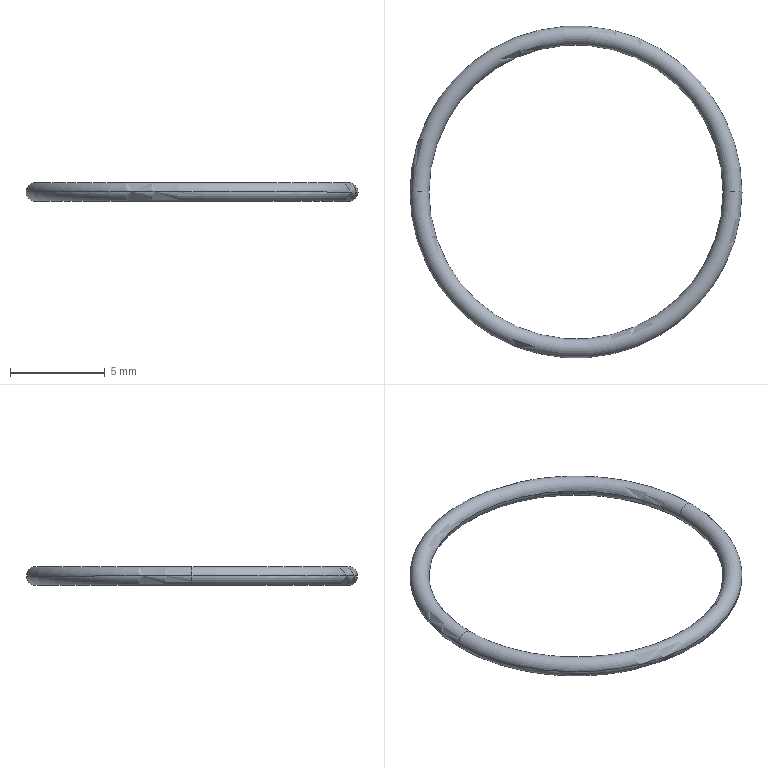Part | SolidWorks | features Sweep 1 | 1 solid | 4 faces | box 17.5 x 17.5 x 1 mm | volume 40.712 mm3 | torus 4
STEP:
#1=CARTESIAN_POINT('',(-8.75,0.,0.));
#2=VERTEX_POINT('',#1);
#3=CARTESIAN_POINT('',(-7.75,0.,0.));
#4=VERTEX_POINT('',#3);
#5=CARTESIAN_POINT('',(-8.25,0.,0.));
#6=DIRECTION('',(0.,1.,0.));
#7=DIRECTION('',(0.,0.,1.));
#8=AXIS2_PLACEMENT_3D('',#5,#6,#7);
#9=CIRCLE('',#8,0.5);
#10=EDGE_CURVE('',#2,#4,#9,.T.);
#11=ORIENTED_EDGE('',*,*,#10,.F.);
#12=CARTESIAN_POINT('',(8.75,0.,0.));
#13=VERTEX_POINT('',#12);
#14=CARTESIAN_POINT('',(0.,0.,0.));
#15=DIRECTION('',(0.,0.,1.));
#16=DIRECTION('',(0.,-1.,0.));
#17=AXIS2_PLACEMENT_3D('',#14,#15,#16);
#18=CIRCLE('',#17,8.75);
#19=EDGE_CURVE('',#2,#13,#18,.T.);
#20=ORIENTED_EDGE('',*,*,#19,.T.);
#21=CARTESIAN_POINT('',(7.75,0.,0.));
#22=VERTEX_POINT('',#21);
#23=CARTESIAN_POINT('',(8.25,0.,0.));
#24=DIRECTION('',(0.,-1.,0.));
#25=DIRECTION('',(0.,0.,-1.));
#26=AXIS2_PLACEMENT_3D('',#23,#24,#25);
#27=CIRCLE('',#26,0.5);
#28=EDGE_CURVE('',#13,#22,#27,.T.);
#29=ORIENTED_EDGE('',*,*,#28,.T.);
#30=CARTESIAN_POINT('',(0.,0.,0.));
#31=DIRECTION('',(0.,0.,1.));
#32=DIRECTION('',(0.,-1.,0.));
#33=AXIS2_PLACEMENT_3D('',#30,#31,#32);
#34=CIRCLE('',#33,7.75);
#35=EDGE_CURVE('',#4,#22,#34,.T.);
#36=ORIENTED_EDGE('',*,*,#35,.F.);
#37=EDGE_LOOP('',(#11,#20,#29,#36));
#38=FACE_OUTER_BOUND('',#37,.T.);
#39=CARTESIAN_POINT('',(0.,0.,0.));
#40=DIRECTION('',(0.,0.,1.));
#41=DIRECTION('',(1.,0.,0.));
#42=AXIS2_PLACEMENT_3D('',#39,#40,#41);
#43=TOROIDAL_SURFACE('',#42,8.25,0.5);
#44=ADVANCED_FACE('',(#38),#43,.T.);
#45=ORIENTED_EDGE('',*,*,#28,.F.);
#46=CARTESIAN_POINT('',(0.,0.,0.));
#47=DIRECTION('',(0.,0.,1.));
#48=DIRECTION('',(0.,-1.,0.));
#49=AXIS2_PLACEMENT_3D('',#46,#47,#48);
#50=CIRCLE('',#49,8.75);
#51=EDGE_CURVE('',#13,#2,#50,.T.);
#52=ORIENTED_EDGE('',*,*,#51,.T.);
#53=ORIENTED_EDGE('',*,*,#10,.T.);
#54=CARTESIAN_POINT('',(0.,0.,0.));
#55=DIRECTION('',(0.,0.,1.));
#56=DIRECTION('',(0.,-1.,0.));
#57=AXIS2_PLACEMENT_3D('',#54,#55,#56);
#58=CIRCLE('',#57,7.75);
#59=EDGE_CURVE('',#22,#4,#58,.T.);
#60=ORIENTED_EDGE('',*,*,#59,.F.);
#61=EDGE_LOOP('',(#45,#52,#53,#60));
#62=FACE_OUTER_BOUND('',#61,.T.);
#63=CARTESIAN_POINT('',(0.,0.,0.));
#64=DIRECTION('',(0.,0.,1.));
#65=DIRECTION('',(1.,0.,0.));
#66=AXIS2_PLACEMENT_3D('',#63,#64,#65);
#67=TOROIDAL_SURFACE('',#66,8.25,0.5);
#68=ADVANCED_FACE('',(#62),#67,.T.);
#69=ORIENTED_EDGE('',*,*,#51,.F.);
#70=CARTESIAN_POINT('',(8.25,0.,0.));
#71=DIRECTION('',(0.,-1.,0.));
#72=DIRECTION('',(0.,0.,-1.));
#73=AXIS2_PLACEMENT_3D('',#70,#71,#72);
#74=CIRCLE('',#73,0.5);
#75=EDGE_CURVE('',#22,#13,#74,.T.);
#76=ORIENTED_EDGE('',*,*,#75,.F.);
#77=ORIENTED_EDGE('',*,*,#59,.T.);
#78=CARTESIAN_POINT('',(-8.25,0.,0.));
#79=DIRECTION('',(0.,1.,0.));
#80=DIRECTION('',(0.,0.,1.));
#81=AXIS2_PLACEMENT_3D('',#78,#79,#80);
#82=CIRCLE('',#81,0.5);
#83=EDGE_CURVE('',#4,#2,#82,.T.);
#84=ORIENTED_EDGE('',*,*,#83,.T.);
#85=EDGE_LOOP('',(#69,#76,#77,#84));
#86=FACE_OUTER_BOUND('',#85,.T.);
#87=CARTESIAN_POINT('',(0.,0.,0.));
#88=DIRECTION('',(0.,0.,1.));
#89=DIRECTION('',(1.,0.,0.));
#90=AXIS2_PLACEMENT_3D('',#87,#88,#89);
#91=TOROIDAL_SURFACE('',#90,8.25,0.5);
#92=ADVANCED_FACE('',(#86),#91,.T.);
#93=ORIENTED_EDGE('',*,*,#19,.F.);
#94=ORIENTED_EDGE('',*,*,#83,.F.);
#95=ORIENTED_EDGE('',*,*,#35,.T.);
#96=ORIENTED_EDGE('',*,*,#75,.T.);
#97=EDGE_LOOP('',(#93,#94,#95,#96));
#98=FACE_OUTER_BOUND('',#97,.T.);
#99=CARTESIAN_POINT('',(0.,0.,0.));
#100=DIRECTION('',(0.,0.,1.));
#101=DIRECTION('',(1.,0.,0.));
#102=AXIS2_PLACEMENT_3D('',#99,#100,#101);
#103=TOROIDAL_SURFACE('',#102,8.25,0.5);
#104=ADVANCED_FACE('',(#98),#103,.T.);
#105=CLOSED_SHELL('',(#44,#68,#92,#104));
#106=MANIFOLD_SOLID_BREP('',#105);
#107=CARTESIAN_POINT('',(0.,0.,0.));
#108=DIRECTION('',(0.,0.,1.));
#109=DIRECTION('',(1.,0.,0.));
#110=AXIS2_PLACEMENT_3D('',#107,#108,#109);
#111=(LENGTH_UNIT()NAMED_UNIT(*)SI_UNIT(.MILLI.,.METRE.));
#112=UNCERTAINTY_MEASURE_WITH_UNIT(LENGTH_MEASURE(0.00001),#111,'','');
#113=(NAMED_UNIT(*)PLANE_ANGLE_UNIT()SI_UNIT($,.RADIAN.));
#114=(NAMED_UNIT(*)SI_UNIT($,.STERADIAN.)SOLID_ANGLE_UNIT());
#115=(GEOMETRIC_REPRESENTATION_CONTEXT(3)GLOBAL_UNCERTAINTY_ASSIGNED_CONTEXT((#112))GLOBAL_UNIT_ASSIGNED_CONTEXT((#111,#113,#114))REPRESENTATION_CONTEXT('',''));
#116=ADVANCED_BREP_SHAPE_REPRESENTATION('',(#106,#110),#115);